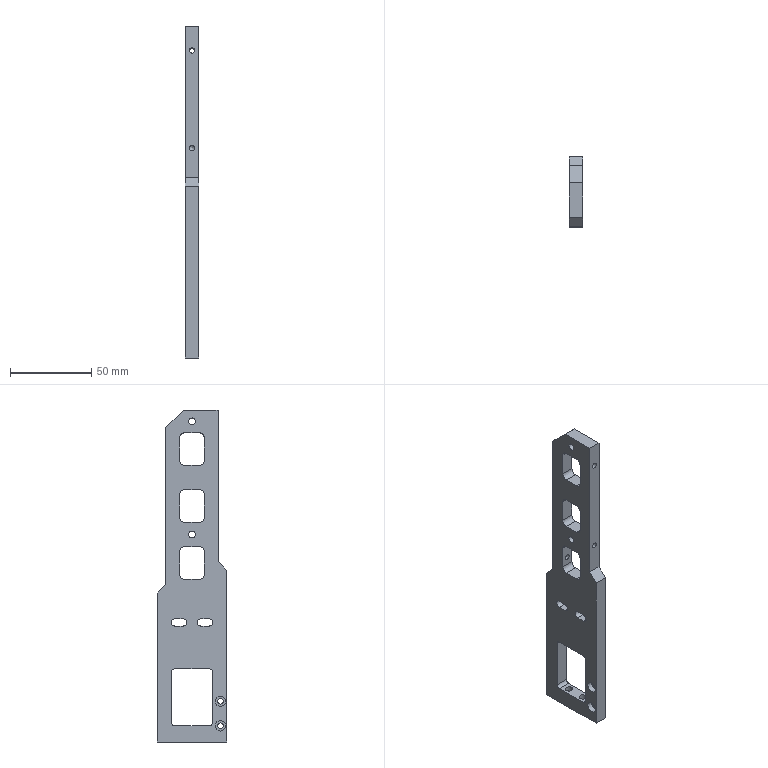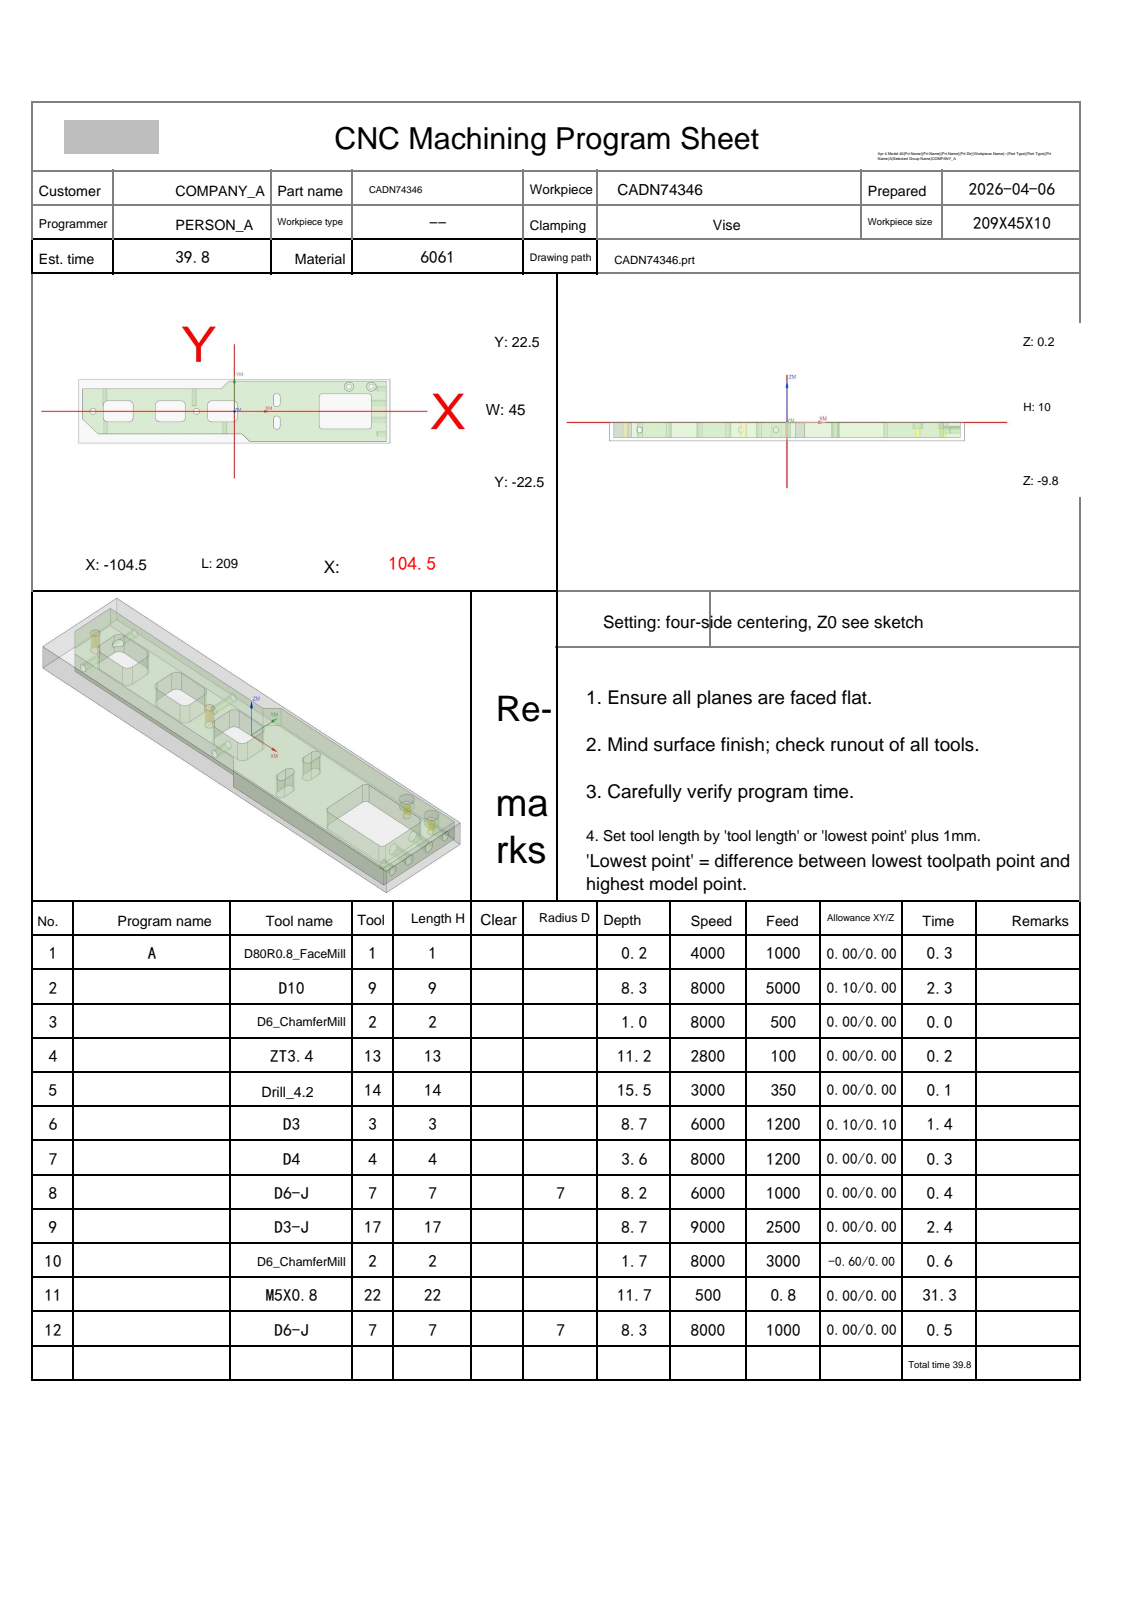NC program | NX | posted by the shop | part box 8 x 43 x 204 mm
Lines 13996 to 14335 of 14335:
N10 T02 M06
(D6_ChamferMill  D=6. R=0. H=02 ce=0.00 di=0.00)
G00 G90 G54 X49. Y23.628 M03 S8000
G43 H02 Z20.
M08
Z2.099
G01 Z-1.5 F3000.
G03 X48.92 Y23.328 I.52 J-.3
X49.22 Y22.808 I.6 J0.0
G01 X49.25 Y22.8
X102.
G02 X103.3 Y21.5 I0.0 J-1.3
G01 Y-21.5
G02 X102. Y-22.8 I-1.3 J0.0
G01 X10.5
X10.246 Y-22.775
X10.003 Y-22.701
X9.778 Y-22.581
X9.581 Y-22.419
X4.462 Y-17.3
X-91.5
X-91.754 Y-17.275
X-91.997 Y-17.201
X-92.222 Y-17.081
X-92.419 Y-16.919
X-102.919 Y-6.419
X-103.081 Y-6.222
X-103.201 Y-5.997
X-103.275 Y-5.754
X-103.3 Y-5.5
Y16.
G02 X-102. Y17.3 I1.3 J0.0
G01 X-9.538
X-4.419 Y22.419
X-4.222 Y22.581
X-3.997 Y22.701
X-3.754 Y22.775
X-3.5 Y22.8
X49.25
X49.28 Y22.808
G03 X49.58 Y23.328 I-.3 J.52
X49.5 Y23.628 I-.6 J0.0
G01 Z2.099
G00 Z20.
X-77.75 Y5.372
Z2.099
G01 Z-1.5
G03 X-77.67 Y5.672 I-.52 J.3
X-77.97 Y6.192 I-.6 J0.0
G01 X-78. Y6.2
X-85.
G03 X-86.7 Y4.5 I0.0 J-1.7
G01 Y-4.5
G03 X-85. Y-6.2 I1.7 J0.0
G01 X-71.
G03 X-69.3 Y-4.5 I0.0 J1.7
G01 Y4.5
G03 X-71. Y6.2 I-1.7 J0.0
G01 X-78.
X-78.03 Y6.192
G03 X-78.33 Y5.672 I.3 J-.52
X-78.25 Y5.372 I.6 J0.0
G01 Z2.099
G00 Z20.
X-42.75
Z2.099
G01 Z-1.5
G03 X-42.67 Y5.672 I-.52 J.3
X-42.97 Y6.192 I-.6 J0.0
G01 X-43. Y6.2
X-50.
G03 X-51.7 Y4.5 I0.0 J-1.7
G01 Y-4.5
G03 X-50. Y-6.2 I1.7 J0.0
G01 X-36.
G03 X-34.3 Y-4.5 I0.0 J1.7
G01 Y4.5
G03 X-36. Y6.2 I-1.7 J0.0
G01 X-43.
X-43.03 Y6.192
G03 X-43.33 Y5.672 I.3 J-.52
X-43.25 Y5.372 I.6 J0.0
G01 Z2.099
G00 Z20.
X-7.75
Z2.099
G01 Z-1.5
G03 X-7.67 Y5.672 I-.52 J.3
X-7.97 Y6.192 I-.6 J0.0
G01 X-8. Y6.2
X-15.
G03 X-16.7 Y4.5 I0.0 J-1.7
G01 Y-4.5
G03 X-15. Y-6.2 I1.7 J0.0
G01 X-1.
G03 X.7 Y-4.5 I0.0 J1.7
G01 Y4.5
G03 X-1. Y6.2 I-1.7 J0.0
G01 X-8.
X-8.03 Y6.192
G03 X-8.33 Y5.672 I.3 J-.52
X-8.25 Y5.372 I.6 J0.0
G01 Z2.099
G00 Z20.
X28.378 Y8.25
Z2.099
G01 Z-1.5
G03 X28.078 Y8.33 I-.3 J-.52
X27.558 Y8.03 I0.0 J-.6
G01 X27.55 Y8.
Y5.5
G03 X28.5 Y4.55 I.95 J0.0
X28.975 Y4.677 I0.0 J.95
G01 X29.172 Y4.828
X29.323 Y5.025
X29.418 Y5.254
X29.45 Y5.5
Y10.5
G03 X28.5 Y11.45 I-.95 J0.0
X28.025 Y11.323 I0.0 J-.95
G01 X27.828 Y11.172
X27.677 Y10.975
X27.582 Y10.746
X27.55 Y10.5
Y8.
X27.558 Y7.97
G03 X28.078 Y7.67 I.52 J.3
X28.378 Y7.75 I0.0 J.6
G01 Z2.099
G00 Z20.
Y-7.75
Z2.099
G01 Z-1.5
G03 X28.078 Y-7.67 I-.3 J-.52
X27.558 Y-7.97 I0.0 J-.6
G01 X27.55 Y-8.
Y-10.5
G03 X28.5 Y-11.45 I.95 J0.0
X28.975 Y-11.323 I0.0 J.95
G01 X29.172 Y-11.172
X29.323 Y-10.975
X29.418 Y-10.746
X29.45 Y-10.5
Y-5.5
G03 X28.5 Y-4.55 I-.95 J0.0
X28.025 Y-4.677 I0.0 J-.95
G01 X27.828 Y-4.828
X27.677 Y-5.025
X27.582 Y-5.254
X27.55 Y-5.5
Y-8.
X27.558 Y-8.03
G03 X28.078 Y-8.33 I.52 J.3
X28.378 Y-8.25 I0.0 J.6
G01 Z2.099
G00 Z20.
X74.25 Y-10.372
Z2.099
G01 Z-1.5
G03 X74.17 Y-10.672 I.52 J-.3
X74.47 Y-11.192 I.6 J0.0
G01 X74.5 Y-11.2
X90.
G03 X90.7 Y-10.5 I0.0 J.7
G01 Y10.5
G03 X90. Y11.2 I-.7 J0.0
G01 X59.
G03 X58.3 Y10.5 I0.0 J-.7
G01 Y-10.5
G03 X59. Y-11.2 I.7 J0.0
G01 X74.5
X74.53 Y-11.192
G03 X74.83 Y-10.672 I-.3 J.52
X74.75 Y-10.372 I-.6 J0.0
G01 Z2.099
G00 Z20.
G00 G90 X-95.093 Y.694 M03 S8000
Z20.
Z-.5
G01 Z-1. F500.
X-95.2 Y1.5
G03 X-96.7 Y0.0 I0.0 J-1.5
X-95. Y-1.7 I1.7 J0.0
X-93.3 Y0.0 I0.0 J1.7
X-95. Y1.7 I-1.7 J0.0
X-96.7 Y0.0 I0.0 J-1.7
X-95.2 Y-1.5 I1.5 J0.0
G01 X-95.093 Y-.694
Z-.5
G00 Z20.
X-25.593 Y.694
Z-.5
G01 Z-1.
X-25.7 Y1.5
G03 X-27.2 Y0.0 I0.0 J-1.5
X-25.5 Y-1.7 I1.7 J0.0
X-23.8 Y0.0 I0.0 J1.7
X-25.5 Y1.7 I-1.7 J0.0
X-27.2 Y0.0 I0.0 J-1.7
X-25.7 Y-1.5 I1.5 J0.0
G01 X-25.593 Y-.694
Z-.5
G00 Z20.
G00 G90 X94.063 Y16.003 M03 S8000
Z20.
Z2.5
G01 X94.108 Y16.06 Z2.474 F500.
X94.281 Y16.353 Z2.35
X94.413 Y16.666 Z2.226
X94.502 Y16.993 Z2.103
X94.547 Y17.33 Z1.979
Y17.67 Z1.855
X94.502 Y18.007 Z1.732
X94.413 Y18.334 Z1.608
X94.281 Y18.647 Z1.484
X94.108 Y18.94 Z1.361
X93.898 Y19.207 Z1.237
X93.655 Y19.444 Z1.113
X93.382 Y19.647 Z.99
X93.168 Y19.77 Z.9
X92.856 Y19.905 Z.776
X92.529 Y19.998 Z.652
X92.193 Y20.046 Z.529
X91.853 Y20.049 Z.405
X91.516 Y20.007 Z.281
X91.188 Y19.92 Z.158
X90.873 Y19.791 Z.034
X90.579 Y19.621 Z-.089
X90.31 Y19.414 Z-.213
X90.071 Y19.172 Z-.337
X89.866 Y18.902 Z-.46
X89.699 Y18.606 Z-.584
X89.572 Y18.29 Z-.708
X89.489 Y17.961 Z-.831
X89.45 Y17.624 Z-.955
Y17.5 Z-1.
G03 X92. Y14.95 I2.55 J0.0
X94.55 Y17.5 I0.0 J2.55
X92. Y20.05 I-2.55 J0.0
X89.45 Y17.5 I0.0 J-2.55
X89.499 Y17.003 I2.55 J0.0
G01 Z1.5
G00 Z20.
X79.063 Y16.003
Z2.5
G01 X79.108 Y16.06 Z2.474
X79.281 Y16.353 Z2.35
X79.413 Y16.666 Z2.226
X79.502 Y16.993 Z2.103
X79.547 Y17.33 Z1.979
Y17.67 Z1.855
X79.502 Y18.007 Z1.732
X79.413 Y18.334 Z1.608
X79.281 Y18.647 Z1.484
X79.108 Y18.94 Z1.361
X78.898 Y19.207 Z1.237
X78.655 Y19.444 Z1.113
X78.382 Y19.647 Z.99
X78.168 Y19.77 Z.9
X77.856 Y19.905 Z.776
X77.529 Y19.998 Z.652
X77.193 Y20.046 Z.529
X76.853 Y20.049 Z.405
X76.516 Y20.007 Z.281
X76.188 Y19.92 Z.158
X75.873 Y19.791 Z.034
X75.579 Y19.621 Z-.089
X75.31 Y19.414 Z-.213
X75.071 Y19.172 Z-.337
X74.866 Y18.902 Z-.46
X74.699 Y18.606 Z-.584
X74.572 Y18.29 Z-.708
X74.489 Y17.961 Z-.831
X74.45 Y17.624 Z-.955
Y17.5 Z-1.
G03 X77. Y14.95 I2.55 J0.0
X79.55 Y17.5 I0.0 J2.55
X77. Y20.05 I-2.55 J0.0
X74.45 Y17.5 I0.0 J-2.55
X74.499 Y17.003 I2.55 J0.0
G01 Z1.5
G00 Z20.
G91 G28 Z0.0
M05
M09
G91 G28 Z0.0
M01
N11 T22 M06
(M5X0.8 D=4.2 DR_a=180 H=22)
G00 G90 G54 X-95. Y0.0 M03 S500
G43 H22 Z20.
M08
G95
G98 G84 X-95. Y0.0 Z-11.5 R1. F.8 Q3.
X-25.5
G80
G94
G00 Z20.
G91 G28 Z0.0
M05
M09
G91 G28 Z0.0
M01
N12 T07 M06
(D6-J  D=6. R=0. H=07 ce=0.00 di=0.00)
G00 G90 G54 X-4.517 Y25.573 M03 S8000
G43 H07 Z20.
M08
Z-7.6
G01 Z-8.1 F1000.
G41 D07
X-4.492 Y25.375
G03 X-3.5 Y24.5 I.992 J.125
G01 X102.
G02 X105. Y21.5 I0.0 J-3.
G01 Y-21.5
G02 X102. Y-24.5 I-3. J0.0
G01 X10.5
G02 X8.379 Y-23.621 I0.0 J3.
G01 X3.757 Y-19.
X-91.5
G02 X-93.621 Y-18.121 I0.0 J3.
G01 X-104.121 Y-7.621
G02 X-105. Y-5.5 I2.121 J2.121
G01 Y16.
G02 X-102. Y19. I3. J0.0
G01 X-10.243
X-5.621 Y23.621
G02 X-3.5 Y24.5 I2.121 J-2.121
G01 X-3.
G03 X-2. Y25.5 I0.0 J1.
G01 G40 Y25.7
Z-7.6
G00 Z20.
M05
M09
G91 G28 Z0.0
G91 G28 Y0.0
M30
%